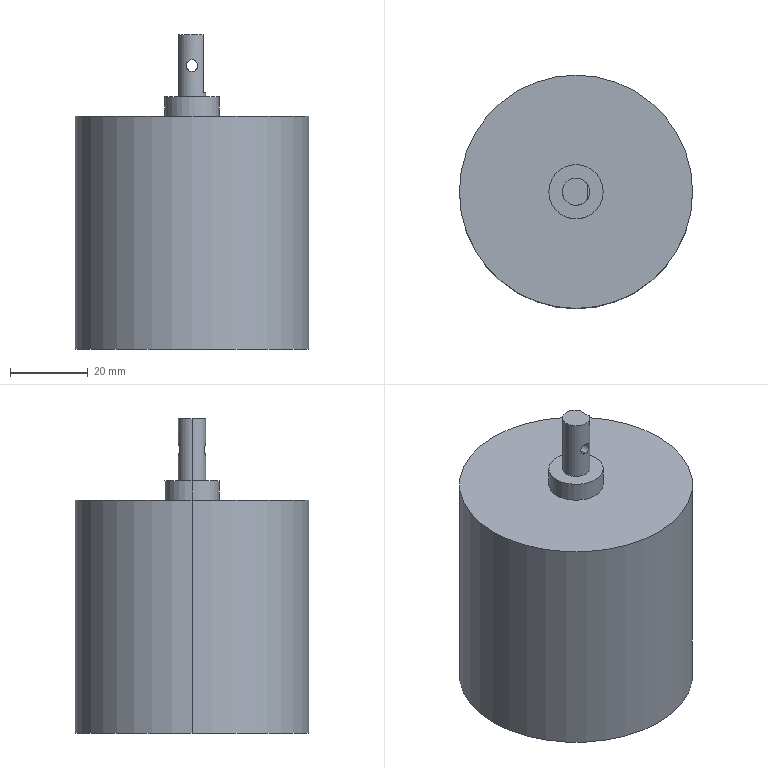Part | SolidWorks | features ICE 4, Extrusion 1 | 1 solid | 14 faces | box 60 x 60 x 81 mm | volume 170965 mm3 | cylinder 8 | plane 6 | commonest cylinder face diameters 3 x2 7 x2 14 x2 60 x2
STEP:
#1=CARTESIAN_POINT('',(0.,3.5,74.5));
#2=VERTEX_POINT('',#1);
#3=CARTESIAN_POINT('',(0.,3.5,71.5));
#4=VERTEX_POINT('',#3);
#5=CARTESIAN_POINT('',(0.,3.5,74.5));
#6=CARTESIAN_POINT('',(-0.09884,3.5,74.5));
#7=CARTESIAN_POINT('',(-0.1992,3.496,74.49));
#8=CARTESIAN_POINT('',(-0.3936,3.479,74.451));
#9=CARTESIAN_POINT('',(-0.4875,3.467,74.422));
#10=CARTESIAN_POINT('',(-0.7601,3.421,74.308));
#11=CARTESIAN_POINT('',(-0.9241,3.379,74.198));
#12=CARTESIAN_POINT('',(-1.13,3.313,73.991));
#13=CARTESIAN_POINT('',(-1.192,3.291,73.916));
#14=CARTESIAN_POINT('',(-1.3,3.25,73.755));
#15=CARTESIAN_POINT('',(-1.347,3.231,73.668));
#16=CARTESIAN_POINT('',(-1.422,3.198,73.487));
#17=CARTESIAN_POINT('',(-1.451,3.185,73.394));
#18=CARTESIAN_POINT('',(-1.49,3.167,73.2));
#19=CARTESIAN_POINT('',(-1.5,3.162,73.099));
#20=CARTESIAN_POINT('',(-1.5,3.162,72.803));
#21=CARTESIAN_POINT('',(-1.46,3.182,72.603));
#22=CARTESIAN_POINT('',(-1.347,3.231,72.332));
#23=CARTESIAN_POINT('',(-1.3,3.25,72.245));
#24=CARTESIAN_POINT('',(-1.192,3.291,72.084));
#25=CARTESIAN_POINT('',(-1.13,3.313,72.009));
#26=CARTESIAN_POINT('',(-0.9236,3.379,71.802));
#27=CARTESIAN_POINT('',(-0.7612,3.421,71.692));
#28=CARTESIAN_POINT('',(-0.3961,3.482,71.54));
#29=CARTESIAN_POINT('',(-0.2007,3.5,71.5));
#30=CARTESIAN_POINT('',(0.,3.5,71.5));
#31=B_SPLINE_CURVE_WITH_KNOTS('',3,(#5,#6,#7,#8,#9,#10,#11,#12,#13,#14,#15,#16,#17,#18,#19,#20,#21,#22,#23,#24,#25,#26,#27,#28,#29,#30),.UNSPECIFIED.,.F.,.F.,(4,2,2,2,2,2,2,2,2,2,2,2,4),(0.004748,0.005044,0.005341,0.005934,0.00623,0.006527,0.006823,0.00712,0.007713,0.008009,0.008306,0.008898,0.009491),.UNSPECIFIED.);
#32=EDGE_CURVE('',#2,#4,#31,.T.);
#33=ORIENTED_EDGE('',*,*,#32,.F.);
#34=CARTESIAN_POINT('',(0.,-3.5,74.5));
#35=VERTEX_POINT('',#34);
#36=CARTESIAN_POINT('',(0.,7.5,74.5));
#37=DIRECTION('',(0.,-1.,0.));
#38=VECTOR('',#37,1000.);
#39=LINE('',#36,#38);
#40=EDGE_CURVE('',#2,#35,#39,.T.);
#41=ORIENTED_EDGE('',*,*,#40,.T.);
#42=CARTESIAN_POINT('',(0.,-3.5,71.5));
#43=VERTEX_POINT('',#42);
#44=CARTESIAN_POINT('',(0.,-3.5,71.5));
#45=CARTESIAN_POINT('',(-0.1004,-3.5,71.5));
#46=CARTESIAN_POINT('',(-0.1989,-3.496,71.51));
#47=CARTESIAN_POINT('',(-0.3924,-3.479,71.549));
#48=CARTESIAN_POINT('',(-0.4883,-3.467,71.578));
#49=CARTESIAN_POINT('',(-0.7602,-3.421,71.692));
#50=CARTESIAN_POINT('',(-0.9249,-3.379,71.803));
#51=CARTESIAN_POINT('',(-1.198,-3.292,72.077));
#52=CARTESIAN_POINT('',(-1.309,-3.247,72.242));
#53=CARTESIAN_POINT('',(-1.422,-3.199,72.512));
#54=CARTESIAN_POINT('',(-1.451,-3.185,72.607));
#55=CARTESIAN_POINT('',(-1.49,-3.167,72.802));
#56=CARTESIAN_POINT('',(-1.5,-3.162,72.9));
#57=CARTESIAN_POINT('',(-1.5,-3.162,73.098));
#58=CARTESIAN_POINT('',(-1.49,-3.167,73.199));
#59=CARTESIAN_POINT('',(-1.451,-3.185,73.392));
#60=CARTESIAN_POINT('',(-1.422,-3.198,73.487));
#61=CARTESIAN_POINT('',(-1.346,-3.231,73.669));
#62=CARTESIAN_POINT('',(-1.3,-3.25,73.755));
#63=CARTESIAN_POINT('',(-1.191,-3.291,73.916));
#64=CARTESIAN_POINT('',(-1.129,-3.314,73.993));
#65=CARTESIAN_POINT('',(-0.9234,-3.379,74.198));
#66=CARTESIAN_POINT('',(-0.758,-3.422,74.309));
#67=CARTESIAN_POINT('',(-0.3976,-3.482,74.459));
#68=CARTESIAN_POINT('',(-0.1979,-3.5,74.5));
#69=CARTESIAN_POINT('',(0.,-3.5,74.5));
#70=B_SPLINE_CURVE_WITH_KNOTS('',3,(#44,#45,#46,#47,#48,#49,#50,#51,#52,#53,#54,#55,#56,#57,#58,#59,#60,#61,#62,#63,#64,#65,#66,#67,#68,#69),.UNSPECIFIED.,.F.,.F.,(4,2,2,2,2,2,2,2,2,2,2,2,4),(0.,0.0002967,0.0005935,0.001187,0.00178,0.002077,0.002374,0.002671,0.002967,0.003264,0.003561,0.004154,0.004748),.UNSPECIFIED.);
#71=EDGE_CURVE('',#43,#35,#70,.T.);
#72=ORIENTED_EDGE('',*,*,#71,.F.);
#73=CARTESIAN_POINT('',(0.,7.5,71.5));
#74=DIRECTION('',(0.,-1.,0.));
#75=VECTOR('',#74,1000.);
#76=LINE('',#73,#75);
#77=EDGE_CURVE('',#4,#43,#76,.T.);
#78=ORIENTED_EDGE('',*,*,#77,.F.);
#79=EDGE_LOOP('',(#33,#41,#72,#78));
#80=FACE_OUTER_BOUND('',#79,.T.);
#81=CARTESIAN_POINT('',(0.,7.5,73.));
#82=DIRECTION('',(0.,-1.,0.));
#83=DIRECTION('',(0.,0.,-1.));
#84=AXIS2_PLACEMENT_3D('',#81,#82,#83);
#85=CYLINDRICAL_SURFACE('',#84,1.5);
#86=ADVANCED_FACE('',(#80),#85,.F.);
#87=CARTESIAN_POINT('',(0.,3.5,71.5));
#88=CARTESIAN_POINT('',(0.1004,3.5,71.5));
#89=CARTESIAN_POINT('',(0.1989,3.496,71.51));
#90=CARTESIAN_POINT('',(0.3924,3.479,71.549));
#91=CARTESIAN_POINT('',(0.4883,3.467,71.578));
#92=CARTESIAN_POINT('',(0.7602,3.421,71.692));
#93=CARTESIAN_POINT('',(0.9249,3.379,71.803));
#94=CARTESIAN_POINT('',(1.198,3.292,72.077));
#95=CARTESIAN_POINT('',(1.309,3.247,72.242));
#96=CARTESIAN_POINT('',(1.422,3.199,72.512));
#97=CARTESIAN_POINT('',(1.451,3.185,72.607));
#98=CARTESIAN_POINT('',(1.49,3.167,72.802));
#99=CARTESIAN_POINT('',(1.5,3.162,72.9));
#100=CARTESIAN_POINT('',(1.5,3.162,73.098));
#101=CARTESIAN_POINT('',(1.49,3.167,73.199));
#102=CARTESIAN_POINT('',(1.451,3.185,73.392));
#103=CARTESIAN_POINT('',(1.422,3.198,73.487));
#104=CARTESIAN_POINT('',(1.346,3.231,73.669));
#105=CARTESIAN_POINT('',(1.3,3.25,73.755));
#106=CARTESIAN_POINT('',(1.191,3.291,73.916));
#107=CARTESIAN_POINT('',(1.129,3.314,73.993));
#108=CARTESIAN_POINT('',(0.9234,3.379,74.198));
#109=CARTESIAN_POINT('',(0.758,3.422,74.309));
#110=CARTESIAN_POINT('',(0.3976,3.482,74.459));
#111=CARTESIAN_POINT('',(0.1979,3.5,74.5));
#112=CARTESIAN_POINT('',(0.,3.5,74.5));
#113=B_SPLINE_CURVE_WITH_KNOTS('',3,(#87,#88,#89,#90,#91,#92,#93,#94,#95,#96,#97,#98,#99,#100,#101,#102,#103,#104,#105,#106,#107,#108,#109,#110,#111,#112),.UNSPECIFIED.,.F.,.F.,(4,2,2,2,2,2,2,2,2,2,2,2,4),(0.,0.0002967,0.0005935,0.001187,0.00178,0.002077,0.002374,0.002671,0.002967,0.003264,0.003561,0.004154,0.004748),.UNSPECIFIED.);
#114=EDGE_CURVE('',#4,#2,#113,.T.);
#115=ORIENTED_EDGE('',*,*,#114,.T.);
#116=ORIENTED_EDGE('',*,*,#32,.T.);
#117=EDGE_LOOP('',(#115,#116));
#118=FACE_BOUND('',#117,.T.);
#119=CARTESIAN_POINT('',(3.5,0.,66.));
#120=VERTEX_POINT('',#119);
#121=CARTESIAN_POINT('',(3.,1.803,66.));
#122=VERTEX_POINT('',#121);
#123=CARTESIAN_POINT('',(0.,0.,66.));
#124=DIRECTION('',(0.,0.,1.));
#125=DIRECTION('',(1.,0.,0.));
#126=AXIS2_PLACEMENT_3D('',#123,#124,#125);
#127=CIRCLE('',#126,3.5);
#128=EDGE_CURVE('',#120,#122,#127,.T.);
#129=ORIENTED_EDGE('',*,*,#128,.F.);
#130=CARTESIAN_POINT('',(3.5,0.,65.));
#131=VERTEX_POINT('',#130);
#132=CARTESIAN_POINT('',(3.5,0.,81.));
#133=DIRECTION('',(0.,0.,-1.));
#134=VECTOR('',#133,1000.);
#135=LINE('',#132,#134);
#136=EDGE_CURVE('',#120,#131,#135,.T.);
#137=ORIENTED_EDGE('',*,*,#136,.T.);
#138=CARTESIAN_POINT('',(-3.5,0.,65.));
#139=VERTEX_POINT('',#138);
#140=CARTESIAN_POINT('',(0.,0.,65.));
#141=DIRECTION('',(0.,0.,1.));
#142=DIRECTION('',(1.,0.,0.));
#143=AXIS2_PLACEMENT_3D('',#140,#141,#142);
#144=CIRCLE('',#143,3.5);
#145=EDGE_CURVE('',#131,#139,#144,.T.);
#146=ORIENTED_EDGE('',*,*,#145,.T.);
#147=CARTESIAN_POINT('',(-3.5,0.,81.));
#148=VERTEX_POINT('',#147);
#149=CARTESIAN_POINT('',(-3.5,0.,81.));
#150=DIRECTION('',(0.,0.,-1.));
#151=VECTOR('',#150,1000.);
#152=LINE('',#149,#151);
#153=EDGE_CURVE('',#148,#139,#152,.T.);
#154=ORIENTED_EDGE('',*,*,#153,.F.);
#155=CARTESIAN_POINT('',(3.,1.803,81.));
#156=VERTEX_POINT('',#155);
#157=CARTESIAN_POINT('',(0.,0.,81.));
#158=DIRECTION('',(0.,0.,1.));
#159=DIRECTION('',(1.,0.,0.));
#160=AXIS2_PLACEMENT_3D('',#157,#158,#159);
#161=CIRCLE('',#160,3.5);
#162=EDGE_CURVE('',#156,#148,#161,.T.);
#163=ORIENTED_EDGE('',*,*,#162,.F.);
#164=CARTESIAN_POINT('',(3.,1.803,66.));
#165=DIRECTION('',(0.,0.,1.));
#166=VECTOR('',#165,1000.);
#167=LINE('',#164,#166);
#168=EDGE_CURVE('',#122,#156,#167,.T.);
#169=ORIENTED_EDGE('',*,*,#168,.F.);
#170=EDGE_LOOP('',(#129,#137,#146,#154,#163,#169));
#171=FACE_OUTER_BOUND('',#170,.T.);
#172=CARTESIAN_POINT('',(0.,0.,81.));
#173=DIRECTION('',(0.,0.,-1.));
#174=DIRECTION('',(-1.,0.,0.));
#175=AXIS2_PLACEMENT_3D('',#172,#173,#174);
#176=CYLINDRICAL_SURFACE('',#175,3.5);
#177=ADVANCED_FACE('',(#118,#171),#176,.T.);
#178=CARTESIAN_POINT('',(7.,0.,65.));
#179=VERTEX_POINT('',#178);
#180=CARTESIAN_POINT('',(-7.,0.,65.));
#181=VERTEX_POINT('',#180);
#182=CARTESIAN_POINT('',(0.,0.,65.));
#183=DIRECTION('',(0.,0.,1.));
#184=DIRECTION('',(1.,0.,0.));
#185=AXIS2_PLACEMENT_3D('',#182,#183,#184);
#186=CIRCLE('',#185,7.);
#187=EDGE_CURVE('',#179,#181,#186,.T.);
#188=ORIENTED_EDGE('',*,*,#187,.F.);
#189=CARTESIAN_POINT('',(7.,0.,60.));
#190=VERTEX_POINT('',#189);
#191=CARTESIAN_POINT('',(7.,0.,65.));
#192=DIRECTION('',(0.,0.,-1.));
#193=VECTOR('',#192,1000.);
#194=LINE('',#191,#193);
#195=EDGE_CURVE('',#179,#190,#194,.T.);
#196=ORIENTED_EDGE('',*,*,#195,.T.);
#197=CARTESIAN_POINT('',(-7.,0.,60.));
#198=VERTEX_POINT('',#197);
#199=CARTESIAN_POINT('',(0.,0.,60.));
#200=DIRECTION('',(0.,0.,1.));
#201=DIRECTION('',(1.,0.,0.));
#202=AXIS2_PLACEMENT_3D('',#199,#200,#201);
#203=CIRCLE('',#202,7.);
#204=EDGE_CURVE('',#190,#198,#203,.T.);
#205=ORIENTED_EDGE('',*,*,#204,.T.);
#206=CARTESIAN_POINT('',(-7.,0.,65.));
#207=DIRECTION('',(0.,0.,-1.));
#208=VECTOR('',#207,1000.);
#209=LINE('',#206,#208);
#210=EDGE_CURVE('',#181,#198,#209,.T.);
#211=ORIENTED_EDGE('',*,*,#210,.F.);
#212=EDGE_LOOP('',(#188,#196,#205,#211));
#213=FACE_OUTER_BOUND('',#212,.T.);
#214=CARTESIAN_POINT('',(0.,0.,65.));
#215=DIRECTION('',(0.,0.,-1.));
#216=DIRECTION('',(-1.,0.,0.));
#217=AXIS2_PLACEMENT_3D('',#214,#215,#216);
#218=CYLINDRICAL_SURFACE('',#217,7.);
#219=ADVANCED_FACE('',(#213),#218,.T.);
#220=CARTESIAN_POINT('',(30.,0.,60.));
#221=VERTEX_POINT('',#220);
#222=CARTESIAN_POINT('',(-30.,0.,60.));
#223=VERTEX_POINT('',#222);
#224=CARTESIAN_POINT('',(0.,0.,60.));
#225=DIRECTION('',(0.,0.,1.));
#226=DIRECTION('',(1.,0.,0.));
#227=AXIS2_PLACEMENT_3D('',#224,#225,#226);
#228=CIRCLE('',#227,30.);
#229=EDGE_CURVE('',#221,#223,#228,.T.);
#230=ORIENTED_EDGE('',*,*,#229,.F.);
#231=CARTESIAN_POINT('',(30.,0.,0.));
#232=VERTEX_POINT('',#231);
#233=CARTESIAN_POINT('',(30.,0.,60.));
#234=DIRECTION('',(0.,0.,-1.));
#235=VECTOR('',#234,1000.);
#236=LINE('',#233,#235);
#237=EDGE_CURVE('',#221,#232,#236,.T.);
#238=ORIENTED_EDGE('',*,*,#237,.T.);
#239=CARTESIAN_POINT('',(-30.,0.,0.));
#240=VERTEX_POINT('',#239);
#241=CARTESIAN_POINT('',(0.,0.,0.));
#242=DIRECTION('',(0.,0.,1.));
#243=DIRECTION('',(1.,0.,0.));
#244=AXIS2_PLACEMENT_3D('',#241,#242,#243);
#245=CIRCLE('',#244,30.);
#246=EDGE_CURVE('',#232,#240,#245,.T.);
#247=ORIENTED_EDGE('',*,*,#246,.T.);
#248=CARTESIAN_POINT('',(-30.,0.,60.));
#249=DIRECTION('',(0.,0.,-1.));
#250=VECTOR('',#249,1000.);
#251=LINE('',#248,#250);
#252=EDGE_CURVE('',#223,#240,#251,.T.);
#253=ORIENTED_EDGE('',*,*,#252,.F.);
#254=EDGE_LOOP('',(#230,#238,#247,#253));
#255=FACE_OUTER_BOUND('',#254,.T.);
#256=CARTESIAN_POINT('',(0.,0.,60.));
#257=DIRECTION('',(0.,0.,-1.));
#258=DIRECTION('',(-1.,0.,0.));
#259=AXIS2_PLACEMENT_3D('',#256,#257,#258);
#260=CYLINDRICAL_SURFACE('',#259,30.);
#261=ADVANCED_FACE('',(#255),#260,.T.);
#262=ORIENTED_EDGE('',*,*,#237,.F.);
#263=CARTESIAN_POINT('',(0.,0.,60.));
#264=DIRECTION('',(0.,0.,1.));
#265=DIRECTION('',(1.,0.,0.));
#266=AXIS2_PLACEMENT_3D('',#263,#264,#265);
#267=CIRCLE('',#266,30.);
#268=EDGE_CURVE('',#223,#221,#267,.T.);
#269=ORIENTED_EDGE('',*,*,#268,.F.);
#270=ORIENTED_EDGE('',*,*,#252,.T.);
#271=CARTESIAN_POINT('',(0.,0.,0.));
#272=DIRECTION('',(0.,0.,1.));
#273=DIRECTION('',(1.,0.,0.));
#274=AXIS2_PLACEMENT_3D('',#271,#272,#273);
#275=CIRCLE('',#274,30.);
#276=EDGE_CURVE('',#240,#232,#275,.T.);
#277=ORIENTED_EDGE('',*,*,#276,.T.);
#278=EDGE_LOOP('',(#262,#269,#270,#277));
#279=FACE_OUTER_BOUND('',#278,.T.);
#280=CARTESIAN_POINT('',(0.,0.,60.));
#281=DIRECTION('',(0.,0.,-1.));
#282=DIRECTION('',(-1.,0.,0.));
#283=AXIS2_PLACEMENT_3D('',#280,#281,#282);
#284=CYLINDRICAL_SURFACE('',#283,30.);
#285=ADVANCED_FACE('',(#279),#284,.T.);
#286=CARTESIAN_POINT('',(0.,0.,60.));
#287=DIRECTION('',(0.,0.,1.));
#288=DIRECTION('',(1.,0.,0.));
#289=AXIS2_PLACEMENT_3D('',#286,#287,#288);
#290=CIRCLE('',#289,7.);
#291=EDGE_CURVE('',#198,#190,#290,.T.);
#292=ORIENTED_EDGE('',*,*,#291,.F.);
#293=ORIENTED_EDGE('',*,*,#204,.F.);
#294=EDGE_LOOP('',(#292,#293));
#295=FACE_BOUND('',#294,.T.);
#296=ORIENTED_EDGE('',*,*,#268,.T.);
#297=ORIENTED_EDGE('',*,*,#229,.T.);
#298=EDGE_LOOP('',(#296,#297));
#299=FACE_OUTER_BOUND('',#298,.T.);
#300=CARTESIAN_POINT('',(0.,0.,60.));
#301=DIRECTION('',(0.,0.,1.));
#302=DIRECTION('',(1.,0.,0.));
#303=AXIS2_PLACEMENT_3D('',#300,#301,#302);
#304=PLANE('',#303);
#305=ADVANCED_FACE('',(#295,#299),#304,.T.);
#306=ORIENTED_EDGE('',*,*,#276,.F.);
#307=ORIENTED_EDGE('',*,*,#246,.F.);
#308=EDGE_LOOP('',(#306,#307));
#309=FACE_OUTER_BOUND('',#308,.T.);
#310=CARTESIAN_POINT('',(0.,0.,0.));
#311=DIRECTION('',(0.,0.,1.));
#312=DIRECTION('',(1.,0.,0.));
#313=AXIS2_PLACEMENT_3D('',#310,#311,#312);
#314=PLANE('',#313);
#315=ADVANCED_FACE('',(#309),#314,.F.);
#316=ORIENTED_EDGE('',*,*,#195,.F.);
#317=CARTESIAN_POINT('',(0.,0.,65.));
#318=DIRECTION('',(0.,0.,1.));
#319=DIRECTION('',(1.,0.,0.));
#320=AXIS2_PLACEMENT_3D('',#317,#318,#319);
#321=CIRCLE('',#320,7.);
#322=EDGE_CURVE('',#181,#179,#321,.T.);
#323=ORIENTED_EDGE('',*,*,#322,.F.);
#324=ORIENTED_EDGE('',*,*,#210,.T.);
#325=ORIENTED_EDGE('',*,*,#291,.T.);
#326=EDGE_LOOP('',(#316,#323,#324,#325));
#327=FACE_OUTER_BOUND('',#326,.T.);
#328=CARTESIAN_POINT('',(0.,0.,65.));
#329=DIRECTION('',(0.,0.,-1.));
#330=DIRECTION('',(-1.,0.,0.));
#331=AXIS2_PLACEMENT_3D('',#328,#329,#330);
#332=CYLINDRICAL_SURFACE('',#331,7.);
#333=ADVANCED_FACE('',(#327),#332,.T.);
#334=CARTESIAN_POINT('',(0.,0.,65.));
#335=DIRECTION('',(0.,0.,1.));
#336=DIRECTION('',(1.,0.,0.));
#337=AXIS2_PLACEMENT_3D('',#334,#335,#336);
#338=CIRCLE('',#337,3.5);
#339=EDGE_CURVE('',#139,#131,#338,.T.);
#340=ORIENTED_EDGE('',*,*,#339,.F.);
#341=ORIENTED_EDGE('',*,*,#145,.F.);
#342=EDGE_LOOP('',(#340,#341));
#343=FACE_BOUND('',#342,.T.);
#344=ORIENTED_EDGE('',*,*,#322,.T.);
#345=ORIENTED_EDGE('',*,*,#187,.T.);
#346=EDGE_LOOP('',(#344,#345));
#347=FACE_OUTER_BOUND('',#346,.T.);
#348=CARTESIAN_POINT('',(0.,0.,65.));
#349=DIRECTION('',(0.,0.,1.));
#350=DIRECTION('',(1.,0.,0.));
#351=AXIS2_PLACEMENT_3D('',#348,#349,#350);
#352=PLANE('',#351);
#353=ADVANCED_FACE('',(#343,#347),#352,.T.);
#354=ORIENTED_EDGE('',*,*,#136,.F.);
#355=CARTESIAN_POINT('',(3.,-1.803,66.));
#356=VERTEX_POINT('',#355);
#357=CARTESIAN_POINT('',(0.,0.,66.));
#358=DIRECTION('',(0.,0.,1.));
#359=DIRECTION('',(1.,0.,0.));
#360=AXIS2_PLACEMENT_3D('',#357,#358,#359);
#361=CIRCLE('',#360,3.5);
#362=EDGE_CURVE('',#356,#120,#361,.T.);
#363=ORIENTED_EDGE('',*,*,#362,.F.);
#364=CARTESIAN_POINT('',(3.,-1.803,81.));
#365=VERTEX_POINT('',#364);
#366=CARTESIAN_POINT('',(3.,-1.803,66.));
#367=DIRECTION('',(0.,0.,1.));
#368=VECTOR('',#367,1000.);
#369=LINE('',#366,#368);
#370=EDGE_CURVE('',#356,#365,#369,.T.);
#371=ORIENTED_EDGE('',*,*,#370,.T.);
#372=CARTESIAN_POINT('',(0.,0.,81.));
#373=DIRECTION('',(0.,0.,1.));
#374=DIRECTION('',(1.,0.,0.));
#375=AXIS2_PLACEMENT_3D('',#372,#373,#374);
#376=CIRCLE('',#375,3.5);
#377=EDGE_CURVE('',#148,#365,#376,.T.);
#378=ORIENTED_EDGE('',*,*,#377,.F.);
#379=ORIENTED_EDGE('',*,*,#153,.T.);
#380=ORIENTED_EDGE('',*,*,#339,.T.);
#381=EDGE_LOOP('',(#354,#363,#371,#378,#379,#380));
#382=FACE_OUTER_BOUND('',#381,.T.);
#383=ORIENTED_EDGE('',*,*,#71,.T.);
#384=CARTESIAN_POINT('',(0.,-3.5,74.5));
#385=CARTESIAN_POINT('',(0.09884,-3.5,74.5));
#386=CARTESIAN_POINT('',(0.1992,-3.496,74.49));
#387=CARTESIAN_POINT('',(0.3936,-3.479,74.451));
#388=CARTESIAN_POINT('',(0.4875,-3.467,74.422));
#389=CARTESIAN_POINT('',(0.7601,-3.421,74.308));
#390=CARTESIAN_POINT('',(0.9241,-3.379,74.198));
#391=CARTESIAN_POINT('',(1.13,-3.313,73.991));
#392=CARTESIAN_POINT('',(1.192,-3.291,73.916));
#393=CARTESIAN_POINT('',(1.3,-3.25,73.755));
#394=CARTESIAN_POINT('',(1.347,-3.231,73.668));
#395=CARTESIAN_POINT('',(1.422,-3.198,73.487));
#396=CARTESIAN_POINT('',(1.451,-3.185,73.394));
#397=CARTESIAN_POINT('',(1.49,-3.167,73.2));
#398=CARTESIAN_POINT('',(1.5,-3.162,73.099));
#399=CARTESIAN_POINT('',(1.5,-3.162,72.803));
#400=CARTESIAN_POINT('',(1.46,-3.182,72.603));
#401=CARTESIAN_POINT('',(1.347,-3.231,72.332));
#402=CARTESIAN_POINT('',(1.3,-3.25,72.245));
#403=CARTESIAN_POINT('',(1.192,-3.291,72.084));
#404=CARTESIAN_POINT('',(1.13,-3.313,72.009));
#405=CARTESIAN_POINT('',(0.9236,-3.379,71.802));
#406=CARTESIAN_POINT('',(0.7612,-3.421,71.692));
#407=CARTESIAN_POINT('',(0.3961,-3.482,71.54));
#408=CARTESIAN_POINT('',(0.2007,-3.5,71.5));
#409=CARTESIAN_POINT('',(0.,-3.5,71.5));
#410=B_SPLINE_CURVE_WITH_KNOTS('',3,(#384,#385,#386,#387,#388,#389,#390,#391,#392,#393,#394,#395,#396,#397,#398,#399,#400,#401,#402,#403,#404,#405,#406,#407,#408,#409),.UNSPECIFIED.,.F.,.F.,(4,2,2,2,2,2,2,2,2,2,2,2,4),(0.004748,0.005044,0.005341,0.005934,0.00623,0.006527,0.006823,0.00712,0.007713,0.008009,0.008306,0.008898,0.009491),.UNSPECIFIED.);
#411=EDGE_CURVE('',#35,#43,#410,.T.);
#412=ORIENTED_EDGE('',*,*,#411,.T.);
#413=EDGE_LOOP('',(#383,#412));
#414=FACE_BOUND('',#413,.T.);
#415=CARTESIAN_POINT('',(0.,0.,81.));
#416=DIRECTION('',(0.,0.,-1.));
#417=DIRECTION('',(-1.,0.,0.));
#418=AXIS2_PLACEMENT_3D('',#415,#416,#417);
#419=CYLINDRICAL_SURFACE('',#418,3.5);
#420=ADVANCED_FACE('',(#382,#414),#419,.T.);
#421=CARTESIAN_POINT('',(3.,0.,81.));
#422=DIRECTION('',(0.,-1.,0.));
#423=VECTOR('',#422,1000.);
#424=LINE('',#421,#423);
#425=EDGE_CURVE('',#156,#365,#424,.T.);
#426=ORIENTED_EDGE('',*,*,#425,.F.);
#427=ORIENTED_EDGE('',*,*,#162,.T.);
#428=ORIENTED_EDGE('',*,*,#377,.T.);
#429=EDGE_LOOP('',(#426,#427,#428));
#430=FACE_OUTER_BOUND('',#429,.T.);
#431=CARTESIAN_POINT('',(0.,0.,81.));
#432=DIRECTION('',(0.,0.,1.));
#433=DIRECTION('',(1.,0.,0.));
#434=AXIS2_PLACEMENT_3D('',#431,#432,#433);
#435=PLANE('',#434);
#436=ADVANCED_FACE('',(#430),#435,.T.);
#437=ORIENTED_EDGE('',*,*,#425,.T.);
#438=ORIENTED_EDGE('',*,*,#370,.F.);
#439=CARTESIAN_POINT('',(3.,0.,66.));
#440=DIRECTION('',(0.,-1.,0.));
#441=VECTOR('',#440,1000.);
#442=LINE('',#439,#441);
#443=EDGE_CURVE('',#122,#356,#442,.T.);
#444=ORIENTED_EDGE('',*,*,#443,.F.);
#445=ORIENTED_EDGE('',*,*,#168,.T.);
#446=EDGE_LOOP('',(#437,#438,#444,#445));
#447=FACE_OUTER_BOUND('',#446,.T.);
#448=CARTESIAN_POINT('',(3.,0.,66.));
#449=DIRECTION('',(-1.,0.,0.));
#450=DIRECTION('',(0.,0.,1.));
#451=AXIS2_PLACEMENT_3D('',#448,#449,#450);
#452=PLANE('',#451);
#453=ADVANCED_FACE('',(#447),#452,.F.);
#454=ORIENTED_EDGE('',*,*,#443,.T.);
#455=ORIENTED_EDGE('',*,*,#362,.T.);
#456=ORIENTED_EDGE('',*,*,#128,.T.);
#457=EDGE_LOOP('',(#454,#455,#456));
#458=FACE_OUTER_BOUND('',#457,.T.);
#459=CARTESIAN_POINT('',(0.,0.,66.));
#460=DIRECTION('',(0.,0.,1.));
#461=DIRECTION('',(1.,0.,0.));
#462=AXIS2_PLACEMENT_3D('',#459,#460,#461);
#463=PLANE('',#462);
#464=ADVANCED_FACE('',(#458),#463,.T.);
#465=ORIENTED_EDGE('',*,*,#40,.F.);
#466=ORIENTED_EDGE('',*,*,#114,.F.);
#467=ORIENTED_EDGE('',*,*,#77,.T.);
#468=ORIENTED_EDGE('',*,*,#411,.F.);
#469=EDGE_LOOP('',(#465,#466,#467,#468));
#470=FACE_OUTER_BOUND('',#469,.T.);
#471=CARTESIAN_POINT('',(0.,7.5,73.));
#472=DIRECTION('',(0.,-1.,0.));
#473=DIRECTION('',(0.,0.,-1.));
#474=AXIS2_PLACEMENT_3D('',#471,#472,#473);
#475=CYLINDRICAL_SURFACE('',#474,1.5);
#476=ADVANCED_FACE('',(#470),#475,.F.);
#477=CLOSED_SHELL('',(#86,#177,#219,#261,#285,#305,#315,#333,#353,#420,#436,#453,#464,#476));
#478=MANIFOLD_SOLID_BREP('',#477);
#479=CARTESIAN_POINT('',(0.,0.,0.));
#480=DIRECTION('',(0.,0.,1.));
#481=DIRECTION('',(1.,0.,0.));
#482=AXIS2_PLACEMENT_3D('',#479,#480,#481);
#483=(LENGTH_UNIT()NAMED_UNIT(*)SI_UNIT(.MILLI.,.METRE.));
#484=UNCERTAINTY_MEASURE_WITH_UNIT(LENGTH_MEASURE(0.00001),#483,'','');
#485=(NAMED_UNIT(*)PLANE_ANGLE_UNIT()SI_UNIT($,.RADIAN.));
#486=(NAMED_UNIT(*)SI_UNIT($,.STERADIAN.)SOLID_ANGLE_UNIT());
#487=(GEOMETRIC_REPRESENTATION_CONTEXT(3)GLOBAL_UNCERTAINTY_ASSIGNED_CONTEXT((#484))GLOBAL_UNIT_ASSIGNED_CONTEXT((#483,#485,#486))REPRESENTATION_CONTEXT('',''));
#488=ADVANCED_BREP_SHAPE_REPRESENTATION('',(#478,#482),#487);